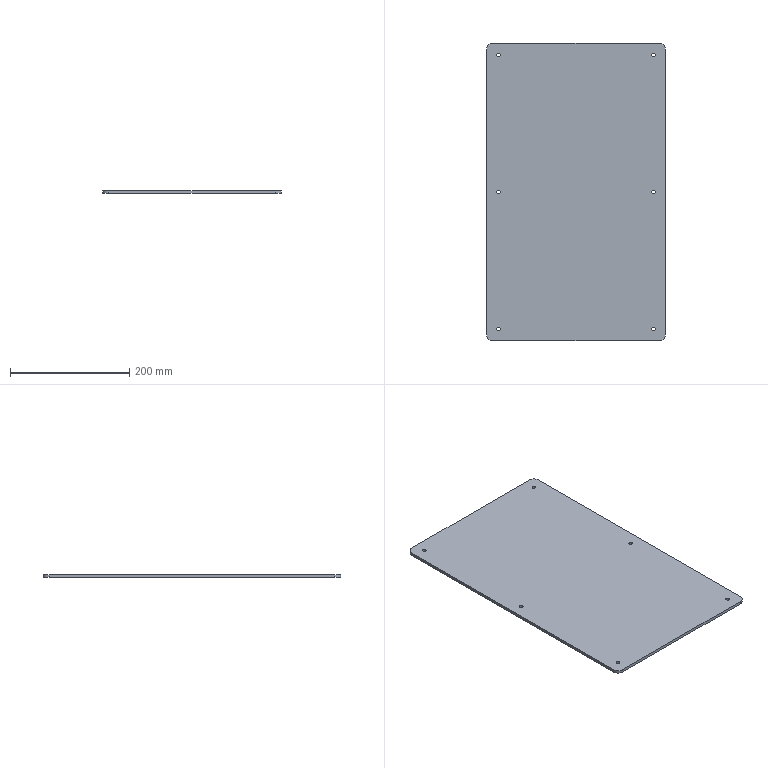Part | SolidWorks | features Extrusion 1, Fillet 1, HoleWzd 1 | 1 solid | 22 faces | box 300 x 500 x 5 mm | volume 748723 mm3 | cylinder 16 | plane 6 | commonest cylinder face diameters 6 x12 20 x4
STEP:
#1=CARTESIAN_POINT('',(-127.,230.,0.));
#2=VERTEX_POINT('',#1);
#3=CARTESIAN_POINT('',(-133.,230.,0.));
#4=VERTEX_POINT('',#3);
#5=CARTESIAN_POINT('',(-130.,230.,0.));
#6=DIRECTION('',(0.,0.,-1.));
#7=DIRECTION('',(-1.,0.,0.));
#8=AXIS2_PLACEMENT_3D('',#5,#6,#7);
#9=CIRCLE('',#8,3.);
#10=EDGE_CURVE('',#2,#4,#9,.T.);
#11=ORIENTED_EDGE('',*,*,#10,.T.);
#12=CARTESIAN_POINT('',(-133.,230.,5.));
#13=VERTEX_POINT('',#12);
#14=CARTESIAN_POINT('',(-133.,230.,5.));
#15=DIRECTION('',(0.,0.,1.));
#16=VECTOR('',#15,1000.);
#17=LINE('',#14,#16);
#18=EDGE_CURVE('',#4,#13,#17,.T.);
#19=ORIENTED_EDGE('',*,*,#18,.T.);
#20=CARTESIAN_POINT('',(-127.,230.,5.));
#21=VERTEX_POINT('',#20);
#22=CARTESIAN_POINT('',(-130.,230.,5.));
#23=DIRECTION('',(0.,0.,1.));
#24=DIRECTION('',(1.,0.,0.));
#25=AXIS2_PLACEMENT_3D('',#22,#23,#24);
#26=CIRCLE('',#25,3.);
#27=EDGE_CURVE('',#13,#21,#26,.T.);
#28=ORIENTED_EDGE('',*,*,#27,.T.);
#29=CARTESIAN_POINT('',(-127.,230.,5.));
#30=DIRECTION('',(0.,0.,1.));
#31=VECTOR('',#30,1000.);
#32=LINE('',#29,#31);
#33=EDGE_CURVE('',#2,#21,#32,.T.);
#34=ORIENTED_EDGE('',*,*,#33,.F.);
#35=EDGE_LOOP('',(#11,#19,#28,#34));
#36=FACE_OUTER_BOUND('',#35,.T.);
#37=CARTESIAN_POINT('',(-130.,230.,5.));
#38=DIRECTION('',(0.,0.,1.));
#39=DIRECTION('',(1.,0.,0.));
#40=AXIS2_PLACEMENT_3D('',#37,#38,#39);
#41=CYLINDRICAL_SURFACE('',#40,3.);
#42=ADVANCED_FACE('',(#36),#41,.F.);
#43=CARTESIAN_POINT('',(133.,230.,0.));
#44=VERTEX_POINT('',#43);
#45=CARTESIAN_POINT('',(127.,230.,0.));
#46=VERTEX_POINT('',#45);
#47=CARTESIAN_POINT('',(130.,230.,0.));
#48=DIRECTION('',(0.,0.,-1.));
#49=DIRECTION('',(-1.,0.,0.));
#50=AXIS2_PLACEMENT_3D('',#47,#48,#49);
#51=CIRCLE('',#50,3.);
#52=EDGE_CURVE('',#44,#46,#51,.T.);
#53=ORIENTED_EDGE('',*,*,#52,.T.);
#54=CARTESIAN_POINT('',(127.,230.,5.));
#55=VERTEX_POINT('',#54);
#56=CARTESIAN_POINT('',(127.,230.,5.));
#57=DIRECTION('',(0.,0.,1.));
#58=VECTOR('',#57,1000.);
#59=LINE('',#56,#58);
#60=EDGE_CURVE('',#46,#55,#59,.T.);
#61=ORIENTED_EDGE('',*,*,#60,.T.);
#62=CARTESIAN_POINT('',(133.,230.,5.));
#63=VERTEX_POINT('',#62);
#64=CARTESIAN_POINT('',(130.,230.,5.));
#65=DIRECTION('',(0.,0.,1.));
#66=DIRECTION('',(1.,0.,0.));
#67=AXIS2_PLACEMENT_3D('',#64,#65,#66);
#68=CIRCLE('',#67,3.);
#69=EDGE_CURVE('',#55,#63,#68,.T.);
#70=ORIENTED_EDGE('',*,*,#69,.T.);
#71=CARTESIAN_POINT('',(133.,230.,5.));
#72=DIRECTION('',(0.,0.,1.));
#73=VECTOR('',#72,1000.);
#74=LINE('',#71,#73);
#75=EDGE_CURVE('',#44,#63,#74,.T.);
#76=ORIENTED_EDGE('',*,*,#75,.F.);
#77=EDGE_LOOP('',(#53,#61,#70,#76));
#78=FACE_OUTER_BOUND('',#77,.T.);
#79=CARTESIAN_POINT('',(130.,230.,5.));
#80=DIRECTION('',(0.,0.,1.));
#81=DIRECTION('',(1.,0.,0.));
#82=AXIS2_PLACEMENT_3D('',#79,#80,#81);
#83=CYLINDRICAL_SURFACE('',#82,3.);
#84=ADVANCED_FACE('',(#78),#83,.F.);
#85=CARTESIAN_POINT('',(133.,-230.,0.));
#86=VERTEX_POINT('',#85);
#87=CARTESIAN_POINT('',(127.,-230.,0.));
#88=VERTEX_POINT('',#87);
#89=CARTESIAN_POINT('',(130.,-230.,0.));
#90=DIRECTION('',(0.,0.,-1.));
#91=DIRECTION('',(-1.,0.,0.));
#92=AXIS2_PLACEMENT_3D('',#89,#90,#91);
#93=CIRCLE('',#92,3.);
#94=EDGE_CURVE('',#86,#88,#93,.T.);
#95=ORIENTED_EDGE('',*,*,#94,.T.);
#96=CARTESIAN_POINT('',(127.,-230.,5.));
#97=VERTEX_POINT('',#96);
#98=CARTESIAN_POINT('',(127.,-230.,5.));
#99=DIRECTION('',(0.,0.,1.));
#100=VECTOR('',#99,1000.);
#101=LINE('',#98,#100);
#102=EDGE_CURVE('',#88,#97,#101,.T.);
#103=ORIENTED_EDGE('',*,*,#102,.T.);
#104=CARTESIAN_POINT('',(133.,-230.,5.));
#105=VERTEX_POINT('',#104);
#106=CARTESIAN_POINT('',(130.,-230.,5.));
#107=DIRECTION('',(0.,0.,1.));
#108=DIRECTION('',(1.,0.,0.));
#109=AXIS2_PLACEMENT_3D('',#106,#107,#108);
#110=CIRCLE('',#109,3.);
#111=EDGE_CURVE('',#97,#105,#110,.T.);
#112=ORIENTED_EDGE('',*,*,#111,.T.);
#113=CARTESIAN_POINT('',(133.,-230.,5.));
#114=DIRECTION('',(0.,0.,1.));
#115=VECTOR('',#114,1000.);
#116=LINE('',#113,#115);
#117=EDGE_CURVE('',#86,#105,#116,.T.);
#118=ORIENTED_EDGE('',*,*,#117,.F.);
#119=EDGE_LOOP('',(#95,#103,#112,#118));
#120=FACE_OUTER_BOUND('',#119,.T.);
#121=CARTESIAN_POINT('',(130.,-230.,5.));
#122=DIRECTION('',(0.,0.,1.));
#123=DIRECTION('',(1.,0.,0.));
#124=AXIS2_PLACEMENT_3D('',#121,#122,#123);
#125=CYLINDRICAL_SURFACE('',#124,3.);
#126=ADVANCED_FACE('',(#120),#125,.F.);
#127=CARTESIAN_POINT('',(-127.,-230.,0.));
#128=VERTEX_POINT('',#127);
#129=CARTESIAN_POINT('',(-133.,-230.,0.));
#130=VERTEX_POINT('',#129);
#131=CARTESIAN_POINT('',(-130.,-230.,0.));
#132=DIRECTION('',(0.,0.,-1.));
#133=DIRECTION('',(-1.,0.,0.));
#134=AXIS2_PLACEMENT_3D('',#131,#132,#133);
#135=CIRCLE('',#134,3.);
#136=EDGE_CURVE('',#128,#130,#135,.T.);
#137=ORIENTED_EDGE('',*,*,#136,.T.);
#138=CARTESIAN_POINT('',(-133.,-230.,5.));
#139=VERTEX_POINT('',#138);
#140=CARTESIAN_POINT('',(-133.,-230.,5.));
#141=DIRECTION('',(0.,0.,1.));
#142=VECTOR('',#141,1000.);
#143=LINE('',#140,#142);
#144=EDGE_CURVE('',#130,#139,#143,.T.);
#145=ORIENTED_EDGE('',*,*,#144,.T.);
#146=CARTESIAN_POINT('',(-127.,-230.,5.));
#147=VERTEX_POINT('',#146);
#148=CARTESIAN_POINT('',(-130.,-230.,5.));
#149=DIRECTION('',(0.,0.,1.));
#150=DIRECTION('',(1.,0.,0.));
#151=AXIS2_PLACEMENT_3D('',#148,#149,#150);
#152=CIRCLE('',#151,3.);
#153=EDGE_CURVE('',#139,#147,#152,.T.);
#154=ORIENTED_EDGE('',*,*,#153,.T.);
#155=CARTESIAN_POINT('',(-127.,-230.,5.));
#156=DIRECTION('',(0.,0.,1.));
#157=VECTOR('',#156,1000.);
#158=LINE('',#155,#157);
#159=EDGE_CURVE('',#128,#147,#158,.T.);
#160=ORIENTED_EDGE('',*,*,#159,.F.);
#161=EDGE_LOOP('',(#137,#145,#154,#160));
#162=FACE_OUTER_BOUND('',#161,.T.);
#163=CARTESIAN_POINT('',(-130.,-230.,5.));
#164=DIRECTION('',(0.,0.,1.));
#165=DIRECTION('',(1.,0.,0.));
#166=AXIS2_PLACEMENT_3D('',#163,#164,#165);
#167=CYLINDRICAL_SURFACE('',#166,3.);
#168=ADVANCED_FACE('',(#162),#167,.F.);
#169=CARTESIAN_POINT('',(-127.,0.,0.));
#170=VERTEX_POINT('',#169);
#171=CARTESIAN_POINT('',(-133.,0.,0.));
#172=VERTEX_POINT('',#171);
#173=CARTESIAN_POINT('',(-130.,0.,0.));
#174=DIRECTION('',(0.,0.,-1.));
#175=DIRECTION('',(-1.,0.,0.));
#176=AXIS2_PLACEMENT_3D('',#173,#174,#175);
#177=CIRCLE('',#176,3.);
#178=EDGE_CURVE('',#170,#172,#177,.T.);
#179=ORIENTED_EDGE('',*,*,#178,.T.);
#180=CARTESIAN_POINT('',(-133.,0.,5.));
#181=VERTEX_POINT('',#180);
#182=CARTESIAN_POINT('',(-133.,0.,5.));
#183=DIRECTION('',(0.,0.,1.));
#184=VECTOR('',#183,1000.);
#185=LINE('',#182,#184);
#186=EDGE_CURVE('',#172,#181,#185,.T.);
#187=ORIENTED_EDGE('',*,*,#186,.T.);
#188=CARTESIAN_POINT('',(-127.,0.,5.));
#189=VERTEX_POINT('',#188);
#190=CARTESIAN_POINT('',(-130.,0.,5.));
#191=DIRECTION('',(0.,0.,1.));
#192=DIRECTION('',(1.,0.,0.));
#193=AXIS2_PLACEMENT_3D('',#190,#191,#192);
#194=CIRCLE('',#193,3.);
#195=EDGE_CURVE('',#181,#189,#194,.T.);
#196=ORIENTED_EDGE('',*,*,#195,.T.);
#197=CARTESIAN_POINT('',(-127.,0.,5.));
#198=DIRECTION('',(0.,0.,1.));
#199=VECTOR('',#198,1000.);
#200=LINE('',#197,#199);
#201=EDGE_CURVE('',#170,#189,#200,.T.);
#202=ORIENTED_EDGE('',*,*,#201,.F.);
#203=EDGE_LOOP('',(#179,#187,#196,#202));
#204=FACE_OUTER_BOUND('',#203,.T.);
#205=CARTESIAN_POINT('',(-130.,0.,5.));
#206=DIRECTION('',(0.,0.,1.));
#207=DIRECTION('',(1.,0.,0.));
#208=AXIS2_PLACEMENT_3D('',#205,#206,#207);
#209=CYLINDRICAL_SURFACE('',#208,3.);
#210=ADVANCED_FACE('',(#204),#209,.F.);
#211=CARTESIAN_POINT('',(133.,0.,0.));
#212=VERTEX_POINT('',#211);
#213=CARTESIAN_POINT('',(127.,0.,0.));
#214=VERTEX_POINT('',#213);
#215=CARTESIAN_POINT('',(130.,0.,0.));
#216=DIRECTION('',(0.,0.,-1.));
#217=DIRECTION('',(-1.,0.,0.));
#218=AXIS2_PLACEMENT_3D('',#215,#216,#217);
#219=CIRCLE('',#218,3.);
#220=EDGE_CURVE('',#212,#214,#219,.T.);
#221=ORIENTED_EDGE('',*,*,#220,.T.);
#222=CARTESIAN_POINT('',(127.,0.,5.));
#223=VERTEX_POINT('',#222);
#224=CARTESIAN_POINT('',(127.,0.,5.));
#225=DIRECTION('',(0.,0.,1.));
#226=VECTOR('',#225,1000.);
#227=LINE('',#224,#226);
#228=EDGE_CURVE('',#214,#223,#227,.T.);
#229=ORIENTED_EDGE('',*,*,#228,.T.);
#230=CARTESIAN_POINT('',(133.,0.,5.));
#231=VERTEX_POINT('',#230);
#232=CARTESIAN_POINT('',(130.,0.,5.));
#233=DIRECTION('',(0.,0.,1.));
#234=DIRECTION('',(1.,0.,0.));
#235=AXIS2_PLACEMENT_3D('',#232,#233,#234);
#236=CIRCLE('',#235,3.);
#237=EDGE_CURVE('',#223,#231,#236,.T.);
#238=ORIENTED_EDGE('',*,*,#237,.T.);
#239=CARTESIAN_POINT('',(133.,0.,5.));
#240=DIRECTION('',(0.,0.,1.));
#241=VECTOR('',#240,1000.);
#242=LINE('',#239,#241);
#243=EDGE_CURVE('',#212,#231,#242,.T.);
#244=ORIENTED_EDGE('',*,*,#243,.F.);
#245=EDGE_LOOP('',(#221,#229,#238,#244));
#246=FACE_OUTER_BOUND('',#245,.T.);
#247=CARTESIAN_POINT('',(130.,0.,5.));
#248=DIRECTION('',(0.,0.,1.));
#249=DIRECTION('',(1.,0.,0.));
#250=AXIS2_PLACEMENT_3D('',#247,#248,#249);
#251=CYLINDRICAL_SURFACE('',#250,3.);
#252=ADVANCED_FACE('',(#246),#251,.F.);
#253=CARTESIAN_POINT('',(150.,-240.,5.));
#254=VERTEX_POINT('',#253);
#255=CARTESIAN_POINT('',(150.,240.,5.));
#256=VERTEX_POINT('',#255);
#257=CARTESIAN_POINT('',(150.,-250.,5.));
#258=DIRECTION('',(0.,1.,0.));
#259=VECTOR('',#258,1000.);
#260=LINE('',#257,#259);
#261=EDGE_CURVE('',#254,#256,#260,.T.);
#262=ORIENTED_EDGE('',*,*,#261,.F.);
#263=CARTESIAN_POINT('',(150.,-240.,0.));
#264=VERTEX_POINT('',#263);
#265=CARTESIAN_POINT('',(150.,-240.,5.));
#266=DIRECTION('',(0.,0.,-1.));
#267=VECTOR('',#266,1000.);
#268=LINE('',#265,#267);
#269=EDGE_CURVE('',#254,#264,#268,.T.);
#270=ORIENTED_EDGE('',*,*,#269,.T.);
#271=CARTESIAN_POINT('',(150.,240.,0.));
#272=VERTEX_POINT('',#271);
#273=CARTESIAN_POINT('',(150.,-250.,0.));
#274=DIRECTION('',(0.,1.,0.));
#275=VECTOR('',#274,1000.);
#276=LINE('',#273,#275);
#277=EDGE_CURVE('',#264,#272,#276,.T.);
#278=ORIENTED_EDGE('',*,*,#277,.T.);
#279=CARTESIAN_POINT('',(150.,240.,5.));
#280=DIRECTION('',(0.,0.,1.));
#281=VECTOR('',#280,1000.);
#282=LINE('',#279,#281);
#283=EDGE_CURVE('',#272,#256,#282,.T.);
#284=ORIENTED_EDGE('',*,*,#283,.T.);
#285=EDGE_LOOP('',(#262,#270,#278,#284));
#286=FACE_OUTER_BOUND('',#285,.T.);
#287=CARTESIAN_POINT('',(150.,-250.,5.));
#288=DIRECTION('',(-1.,0.,0.));
#289=DIRECTION('',(0.,0.,1.));
#290=AXIS2_PLACEMENT_3D('',#287,#288,#289);
#291=PLANE('',#290);
#292=ADVANCED_FACE('',(#286),#291,.F.);
#293=CARTESIAN_POINT('',(140.,250.,5.));
#294=VERTEX_POINT('',#293);
#295=CARTESIAN_POINT('',(-140.,250.,5.));
#296=VERTEX_POINT('',#295);
#297=CARTESIAN_POINT('',(-150.,250.,5.));
#298=DIRECTION('',(-1.,0.,0.));
#299=VECTOR('',#298,1000.);
#300=LINE('',#297,#299);
#301=EDGE_CURVE('',#294,#296,#300,.T.);
#302=ORIENTED_EDGE('',*,*,#301,.F.);
#303=CARTESIAN_POINT('',(140.,250.,0.));
#304=VERTEX_POINT('',#303);
#305=CARTESIAN_POINT('',(140.,250.,5.));
#306=DIRECTION('',(0.,0.,-1.));
#307=VECTOR('',#306,1000.);
#308=LINE('',#305,#307);
#309=EDGE_CURVE('',#294,#304,#308,.T.);
#310=ORIENTED_EDGE('',*,*,#309,.T.);
#311=CARTESIAN_POINT('',(-140.,250.,0.));
#312=VERTEX_POINT('',#311);
#313=CARTESIAN_POINT('',(-150.,250.,0.));
#314=DIRECTION('',(-1.,0.,0.));
#315=VECTOR('',#314,1000.);
#316=LINE('',#313,#315);
#317=EDGE_CURVE('',#304,#312,#316,.T.);
#318=ORIENTED_EDGE('',*,*,#317,.T.);
#319=CARTESIAN_POINT('',(-140.,250.,5.));
#320=DIRECTION('',(0.,0.,1.));
#321=VECTOR('',#320,1000.);
#322=LINE('',#319,#321);
#323=EDGE_CURVE('',#312,#296,#322,.T.);
#324=ORIENTED_EDGE('',*,*,#323,.T.);
#325=EDGE_LOOP('',(#302,#310,#318,#324));
#326=FACE_OUTER_BOUND('',#325,.T.);
#327=CARTESIAN_POINT('',(-150.,250.,5.));
#328=DIRECTION('',(0.,-1.,0.));
#329=DIRECTION('',(0.,0.,-1.));
#330=AXIS2_PLACEMENT_3D('',#327,#328,#329);
#331=PLANE('',#330);
#332=ADVANCED_FACE('',(#326),#331,.F.);
#333=CARTESIAN_POINT('',(-150.,240.,0.));
#334=VERTEX_POINT('',#333);
#335=CARTESIAN_POINT('',(-150.,-240.,0.));
#336=VERTEX_POINT('',#335);
#337=CARTESIAN_POINT('',(-150.,-250.,0.));
#338=DIRECTION('',(0.,-1.,0.));
#339=VECTOR('',#338,1000.);
#340=LINE('',#337,#339);
#341=EDGE_CURVE('',#334,#336,#340,.T.);
#342=ORIENTED_EDGE('',*,*,#341,.T.);
#343=CARTESIAN_POINT('',(-150.,-240.,5.));
#344=VERTEX_POINT('',#343);
#345=CARTESIAN_POINT('',(-150.,-240.,5.));
#346=DIRECTION('',(0.,0.,1.));
#347=VECTOR('',#346,1000.);
#348=LINE('',#345,#347);
#349=EDGE_CURVE('',#336,#344,#348,.T.);
#350=ORIENTED_EDGE('',*,*,#349,.T.);
#351=CARTESIAN_POINT('',(-150.,240.,5.));
#352=VERTEX_POINT('',#351);
#353=CARTESIAN_POINT('',(-150.,-250.,5.));
#354=DIRECTION('',(0.,-1.,0.));
#355=VECTOR('',#354,1000.);
#356=LINE('',#353,#355);
#357=EDGE_CURVE('',#352,#344,#356,.T.);
#358=ORIENTED_EDGE('',*,*,#357,.F.);
#359=CARTESIAN_POINT('',(-150.,240.,5.));
#360=DIRECTION('',(0.,0.,-1.));
#361=VECTOR('',#360,1000.);
#362=LINE('',#359,#361);
#363=EDGE_CURVE('',#352,#334,#362,.T.);
#364=ORIENTED_EDGE('',*,*,#363,.T.);
#365=EDGE_LOOP('',(#342,#350,#358,#364));
#366=FACE_OUTER_BOUND('',#365,.T.);
#367=CARTESIAN_POINT('',(-150.,-250.,5.));
#368=DIRECTION('',(1.,0.,0.));
#369=DIRECTION('',(0.,0.,-1.));
#370=AXIS2_PLACEMENT_3D('',#367,#368,#369);
#371=PLANE('',#370);
#372=ADVANCED_FACE('',(#366),#371,.F.);
#373=CARTESIAN_POINT('',(-140.,-250.,5.));
#374=VERTEX_POINT('',#373);
#375=CARTESIAN_POINT('',(140.,-250.,5.));
#376=VERTEX_POINT('',#375);
#377=CARTESIAN_POINT('',(-150.,-250.,5.));
#378=DIRECTION('',(1.,0.,0.));
#379=VECTOR('',#378,1000.);
#380=LINE('',#377,#379);
#381=EDGE_CURVE('',#374,#376,#380,.T.);
#382=ORIENTED_EDGE('',*,*,#381,.F.);
#383=CARTESIAN_POINT('',(-140.,-250.,0.));
#384=VERTEX_POINT('',#383);
#385=CARTESIAN_POINT('',(-140.,-250.,5.));
#386=DIRECTION('',(0.,0.,-1.));
#387=VECTOR('',#386,1000.);
#388=LINE('',#385,#387);
#389=EDGE_CURVE('',#374,#384,#388,.T.);
#390=ORIENTED_EDGE('',*,*,#389,.T.);
#391=CARTESIAN_POINT('',(140.,-250.,0.));
#392=VERTEX_POINT('',#391);
#393=CARTESIAN_POINT('',(-150.,-250.,0.));
#394=DIRECTION('',(1.,0.,0.));
#395=VECTOR('',#394,1000.);
#396=LINE('',#393,#395);
#397=EDGE_CURVE('',#384,#392,#396,.T.);
#398=ORIENTED_EDGE('',*,*,#397,.T.);
#399=CARTESIAN_POINT('',(140.,-250.,5.));
#400=DIRECTION('',(0.,0.,1.));
#401=VECTOR('',#400,1000.);
#402=LINE('',#399,#401);
#403=EDGE_CURVE('',#392,#376,#402,.T.);
#404=ORIENTED_EDGE('',*,*,#403,.T.);
#405=EDGE_LOOP('',(#382,#390,#398,#404));
#406=FACE_OUTER_BOUND('',#405,.T.);
#407=CARTESIAN_POINT('',(-150.,-250.,5.));
#408=DIRECTION('',(0.,1.,0.));
#409=DIRECTION('',(0.,0.,1.));
#410=AXIS2_PLACEMENT_3D('',#407,#408,#409);
#411=PLANE('',#410);
#412=ADVANCED_FACE('',(#406),#411,.F.);
#413=CARTESIAN_POINT('',(-130.,230.,5.));
#414=DIRECTION('',(0.,0.,1.));
#415=DIRECTION('',(1.,0.,0.));
#416=AXIS2_PLACEMENT_3D('',#413,#414,#415);
#417=CIRCLE('',#416,3.);
#418=EDGE_CURVE('',#21,#13,#417,.T.);
#419=ORIENTED_EDGE('',*,*,#418,.F.);
#420=ORIENTED_EDGE('',*,*,#27,.F.);
#421=EDGE_LOOP('',(#419,#420));
#422=FACE_BOUND('',#421,.T.);
#423=CARTESIAN_POINT('',(130.,230.,5.));
#424=DIRECTION('',(0.,0.,1.));
#425=DIRECTION('',(1.,0.,0.));
#426=AXIS2_PLACEMENT_3D('',#423,#424,#425);
#427=CIRCLE('',#426,3.);
#428=EDGE_CURVE('',#63,#55,#427,.T.);
#429=ORIENTED_EDGE('',*,*,#428,.F.);
#430=ORIENTED_EDGE('',*,*,#69,.F.);
#431=EDGE_LOOP('',(#429,#430));
#432=FACE_BOUND('',#431,.T.);
#433=CARTESIAN_POINT('',(130.,-230.,5.));
#434=DIRECTION('',(0.,0.,1.));
#435=DIRECTION('',(1.,0.,0.));
#436=AXIS2_PLACEMENT_3D('',#433,#434,#435);
#437=CIRCLE('',#436,3.);
#438=EDGE_CURVE('',#105,#97,#437,.T.);
#439=ORIENTED_EDGE('',*,*,#438,.F.);
#440=ORIENTED_EDGE('',*,*,#111,.F.);
#441=EDGE_LOOP('',(#439,#440));
#442=FACE_BOUND('',#441,.T.);
#443=CARTESIAN_POINT('',(-130.,-230.,5.));
#444=DIRECTION('',(0.,0.,1.));
#445=DIRECTION('',(1.,0.,0.));
#446=AXIS2_PLACEMENT_3D('',#443,#444,#445);
#447=CIRCLE('',#446,3.);
#448=EDGE_CURVE('',#147,#139,#447,.T.);
#449=ORIENTED_EDGE('',*,*,#448,.F.);
#450=ORIENTED_EDGE('',*,*,#153,.F.);
#451=EDGE_LOOP('',(#449,#450));
#452=FACE_BOUND('',#451,.T.);
#453=CARTESIAN_POINT('',(-130.,0.,5.));
#454=DIRECTION('',(0.,0.,1.));
#455=DIRECTION('',(1.,0.,0.));
#456=AXIS2_PLACEMENT_3D('',#453,#454,#455);
#457=CIRCLE('',#456,3.);
#458=EDGE_CURVE('',#189,#181,#457,.T.);
#459=ORIENTED_EDGE('',*,*,#458,.F.);
#460=ORIENTED_EDGE('',*,*,#195,.F.);
#461=EDGE_LOOP('',(#459,#460));
#462=FACE_BOUND('',#461,.T.);
#463=CARTESIAN_POINT('',(130.,0.,5.));
#464=DIRECTION('',(0.,0.,1.));
#465=DIRECTION('',(1.,0.,0.));
#466=AXIS2_PLACEMENT_3D('',#463,#464,#465);
#467=CIRCLE('',#466,3.);
#468=EDGE_CURVE('',#231,#223,#467,.T.);
#469=ORIENTED_EDGE('',*,*,#468,.F.);
#470=ORIENTED_EDGE('',*,*,#237,.F.);
#471=EDGE_LOOP('',(#469,#470));
#472=FACE_BOUND('',#471,.T.);
#473=ORIENTED_EDGE('',*,*,#357,.T.);
#474=CARTESIAN_POINT('',(-140.,-240.,5.));
#475=DIRECTION('',(0.,0.,1.));
#476=DIRECTION('',(-1.,0.,0.));
#477=AXIS2_PLACEMENT_3D('',#474,#475,#476);
#478=CIRCLE('',#477,10.);
#479=EDGE_CURVE('',#344,#374,#478,.T.);
#480=ORIENTED_EDGE('',*,*,#479,.T.);
#481=ORIENTED_EDGE('',*,*,#381,.T.);
#482=CARTESIAN_POINT('',(140.,-240.,5.));
#483=DIRECTION('',(0.,0.,1.));
#484=DIRECTION('',(-1.,0.,0.));
#485=AXIS2_PLACEMENT_3D('',#482,#483,#484);
#486=CIRCLE('',#485,10.);
#487=EDGE_CURVE('',#376,#254,#486,.T.);
#488=ORIENTED_EDGE('',*,*,#487,.T.);
#489=ORIENTED_EDGE('',*,*,#261,.T.);
#490=CARTESIAN_POINT('',(140.,240.,5.));
#491=DIRECTION('',(0.,0.,1.));
#492=DIRECTION('',(-1.,0.,0.));
#493=AXIS2_PLACEMENT_3D('',#490,#491,#492);
#494=CIRCLE('',#493,10.);
#495=EDGE_CURVE('',#256,#294,#494,.T.);
#496=ORIENTED_EDGE('',*,*,#495,.T.);
#497=ORIENTED_EDGE('',*,*,#301,.T.);
#498=CARTESIAN_POINT('',(-140.,240.,5.));
#499=DIRECTION('',(0.,0.,1.));
#500=DIRECTION('',(-1.,0.,0.));
#501=AXIS2_PLACEMENT_3D('',#498,#499,#500);
#502=CIRCLE('',#501,10.);
#503=EDGE_CURVE('',#296,#352,#502,.T.);
#504=ORIENTED_EDGE('',*,*,#503,.T.);
#505=EDGE_LOOP('',(#473,#480,#481,#488,#489,#496,#497,#504));
#506=FACE_OUTER_BOUND('',#505,.T.);
#507=CARTESIAN_POINT('',(0.,0.,5.));
#508=DIRECTION('',(0.,0.,-1.));
#509=DIRECTION('',(-1.,0.,0.));
#510=AXIS2_PLACEMENT_3D('',#507,#508,#509);
#511=PLANE('',#510);
#512=ADVANCED_FACE('',(#422,#432,#442,#452,#462,#472,#506),#511,.F.);
#513=ORIENTED_EDGE('',*,*,#10,.F.);
#514=CARTESIAN_POINT('',(-130.,230.,0.));
#515=DIRECTION('',(0.,0.,-1.));
#516=DIRECTION('',(-1.,0.,0.));
#517=AXIS2_PLACEMENT_3D('',#514,#515,#516);
#518=CIRCLE('',#517,3.);
#519=EDGE_CURVE('',#4,#2,#518,.T.);
#520=ORIENTED_EDGE('',*,*,#519,.F.);
#521=EDGE_LOOP('',(#513,#520));
#522=FACE_BOUND('',#521,.T.);
#523=ORIENTED_EDGE('',*,*,#52,.F.);
#524=CARTESIAN_POINT('',(130.,230.,0.));
#525=DIRECTION('',(0.,0.,-1.));
#526=DIRECTION('',(-1.,0.,0.));
#527=AXIS2_PLACEMENT_3D('',#524,#525,#526);
#528=CIRCLE('',#527,3.);
#529=EDGE_CURVE('',#46,#44,#528,.T.);
#530=ORIENTED_EDGE('',*,*,#529,.F.);
#531=EDGE_LOOP('',(#523,#530));
#532=FACE_BOUND('',#531,.T.);
#533=ORIENTED_EDGE('',*,*,#94,.F.);
#534=CARTESIAN_POINT('',(130.,-230.,0.));
#535=DIRECTION('',(0.,0.,-1.));
#536=DIRECTION('',(-1.,0.,0.));
#537=AXIS2_PLACEMENT_3D('',#534,#535,#536);
#538=CIRCLE('',#537,3.);
#539=EDGE_CURVE('',#88,#86,#538,.T.);
#540=ORIENTED_EDGE('',*,*,#539,.F.);
#541=EDGE_LOOP('',(#533,#540));
#542=FACE_BOUND('',#541,.T.);
#543=ORIENTED_EDGE('',*,*,#136,.F.);
#544=CARTESIAN_POINT('',(-130.,-230.,0.));
#545=DIRECTION('',(0.,0.,-1.));
#546=DIRECTION('',(-1.,0.,0.));
#547=AXIS2_PLACEMENT_3D('',#544,#545,#546);
#548=CIRCLE('',#547,3.);
#549=EDGE_CURVE('',#130,#128,#548,.T.);
#550=ORIENTED_EDGE('',*,*,#549,.F.);
#551=EDGE_LOOP('',(#543,#550));
#552=FACE_BOUND('',#551,.T.);
#553=ORIENTED_EDGE('',*,*,#178,.F.);
#554=CARTESIAN_POINT('',(-130.,0.,0.));
#555=DIRECTION('',(0.,0.,-1.));
#556=DIRECTION('',(-1.,0.,0.));
#557=AXIS2_PLACEMENT_3D('',#554,#555,#556);
#558=CIRCLE('',#557,3.);
#559=EDGE_CURVE('',#172,#170,#558,.T.);
#560=ORIENTED_EDGE('',*,*,#559,.F.);
#561=EDGE_LOOP('',(#553,#560));
#562=FACE_BOUND('',#561,.T.);
#563=ORIENTED_EDGE('',*,*,#220,.F.);
#564=CARTESIAN_POINT('',(130.,0.,0.));
#565=DIRECTION('',(0.,0.,-1.));
#566=DIRECTION('',(-1.,0.,0.));
#567=AXIS2_PLACEMENT_3D('',#564,#565,#566);
#568=CIRCLE('',#567,3.);
#569=EDGE_CURVE('',#214,#212,#568,.T.);
#570=ORIENTED_EDGE('',*,*,#569,.F.);
#571=EDGE_LOOP('',(#563,#570));
#572=FACE_BOUND('',#571,.T.);
#573=ORIENTED_EDGE('',*,*,#397,.F.);
#574=CARTESIAN_POINT('',(-140.,-240.,0.));
#575=DIRECTION('',(0.,0.,-1.));
#576=DIRECTION('',(-1.,0.,0.));
#577=AXIS2_PLACEMENT_3D('',#574,#575,#576);
#578=CIRCLE('',#577,10.);
#579=EDGE_CURVE('',#384,#336,#578,.T.);
#580=ORIENTED_EDGE('',*,*,#579,.T.);
#581=ORIENTED_EDGE('',*,*,#341,.F.);
#582=CARTESIAN_POINT('',(-140.,240.,0.));
#583=DIRECTION('',(0.,0.,-1.));
#584=DIRECTION('',(-1.,0.,0.));
#585=AXIS2_PLACEMENT_3D('',#582,#583,#584);
#586=CIRCLE('',#585,10.);
#587=EDGE_CURVE('',#334,#312,#586,.T.);
#588=ORIENTED_EDGE('',*,*,#587,.T.);
#589=ORIENTED_EDGE('',*,*,#317,.F.);
#590=CARTESIAN_POINT('',(140.,240.,0.));
#591=DIRECTION('',(0.,0.,-1.));
#592=DIRECTION('',(-1.,0.,0.));
#593=AXIS2_PLACEMENT_3D('',#590,#591,#592);
#594=CIRCLE('',#593,10.);
#595=EDGE_CURVE('',#304,#272,#594,.T.);
#596=ORIENTED_EDGE('',*,*,#595,.T.);
#597=ORIENTED_EDGE('',*,*,#277,.F.);
#598=CARTESIAN_POINT('',(140.,-240.,0.));
#599=DIRECTION('',(0.,0.,-1.));
#600=DIRECTION('',(-1.,0.,0.));
#601=AXIS2_PLACEMENT_3D('',#598,#599,#600);
#602=CIRCLE('',#601,10.);
#603=EDGE_CURVE('',#264,#392,#602,.T.);
#604=ORIENTED_EDGE('',*,*,#603,.T.);
#605=EDGE_LOOP('',(#573,#580,#581,#588,#589,#596,#597,#604));
#606=FACE_OUTER_BOUND('',#605,.T.);
#607=CARTESIAN_POINT('',(0.,0.,0.));
#608=DIRECTION('',(0.,0.,-1.));
#609=DIRECTION('',(-1.,0.,0.));
#610=AXIS2_PLACEMENT_3D('',#607,#608,#609);
#611=PLANE('',#610);
#612=ADVANCED_FACE('',(#522,#532,#542,#552,#562,#572,#606),#611,.T.);
#613=ORIENTED_EDGE('',*,*,#228,.F.);
#614=ORIENTED_EDGE('',*,*,#569,.T.);
#615=ORIENTED_EDGE('',*,*,#243,.T.);
#616=ORIENTED_EDGE('',*,*,#468,.T.);
#617=EDGE_LOOP('',(#613,#614,#615,#616));
#618=FACE_OUTER_BOUND('',#617,.T.);
#619=CARTESIAN_POINT('',(130.,0.,5.));
#620=DIRECTION('',(0.,0.,1.));
#621=DIRECTION('',(1.,0.,0.));
#622=AXIS2_PLACEMENT_3D('',#619,#620,#621);
#623=CYLINDRICAL_SURFACE('',#622,3.);
#624=ADVANCED_FACE('',(#618),#623,.F.);
#625=ORIENTED_EDGE('',*,*,#186,.F.);
#626=ORIENTED_EDGE('',*,*,#559,.T.);
#627=ORIENTED_EDGE('',*,*,#201,.T.);
#628=ORIENTED_EDGE('',*,*,#458,.T.);
#629=EDGE_LOOP('',(#625,#626,#627,#628));
#630=FACE_OUTER_BOUND('',#629,.T.);
#631=CARTESIAN_POINT('',(-130.,0.,5.));
#632=DIRECTION('',(0.,0.,1.));
#633=DIRECTION('',(1.,0.,0.));
#634=AXIS2_PLACEMENT_3D('',#631,#632,#633);
#635=CYLINDRICAL_SURFACE('',#634,3.);
#636=ADVANCED_FACE('',(#630),#635,.F.);
#637=ORIENTED_EDGE('',*,*,#144,.F.);
#638=ORIENTED_EDGE('',*,*,#549,.T.);
#639=ORIENTED_EDGE('',*,*,#159,.T.);
#640=ORIENTED_EDGE('',*,*,#448,.T.);
#641=EDGE_LOOP('',(#637,#638,#639,#640));
#642=FACE_OUTER_BOUND('',#641,.T.);
#643=CARTESIAN_POINT('',(-130.,-230.,5.));
#644=DIRECTION('',(0.,0.,1.));
#645=DIRECTION('',(1.,0.,0.));
#646=AXIS2_PLACEMENT_3D('',#643,#644,#645);
#647=CYLINDRICAL_SURFACE('',#646,3.);
#648=ADVANCED_FACE('',(#642),#647,.F.);
#649=ORIENTED_EDGE('',*,*,#102,.F.);
#650=ORIENTED_EDGE('',*,*,#539,.T.);
#651=ORIENTED_EDGE('',*,*,#117,.T.);
#652=ORIENTED_EDGE('',*,*,#438,.T.);
#653=EDGE_LOOP('',(#649,#650,#651,#652));
#654=FACE_OUTER_BOUND('',#653,.T.);
#655=CARTESIAN_POINT('',(130.,-230.,5.));
#656=DIRECTION('',(0.,0.,1.));
#657=DIRECTION('',(1.,0.,0.));
#658=AXIS2_PLACEMENT_3D('',#655,#656,#657);
#659=CYLINDRICAL_SURFACE('',#658,3.);
#660=ADVANCED_FACE('',(#654),#659,.F.);
#661=ORIENTED_EDGE('',*,*,#60,.F.);
#662=ORIENTED_EDGE('',*,*,#529,.T.);
#663=ORIENTED_EDGE('',*,*,#75,.T.);
#664=ORIENTED_EDGE('',*,*,#428,.T.);
#665=EDGE_LOOP('',(#661,#662,#663,#664));
#666=FACE_OUTER_BOUND('',#665,.T.);
#667=CARTESIAN_POINT('',(130.,230.,5.));
#668=DIRECTION('',(0.,0.,1.));
#669=DIRECTION('',(1.,0.,0.));
#670=AXIS2_PLACEMENT_3D('',#667,#668,#669);
#671=CYLINDRICAL_SURFACE('',#670,3.);
#672=ADVANCED_FACE('',(#666),#671,.F.);
#673=ORIENTED_EDGE('',*,*,#18,.F.);
#674=ORIENTED_EDGE('',*,*,#519,.T.);
#675=ORIENTED_EDGE('',*,*,#33,.T.);
#676=ORIENTED_EDGE('',*,*,#418,.T.);
#677=EDGE_LOOP('',(#673,#674,#675,#676));
#678=FACE_OUTER_BOUND('',#677,.T.);
#679=CARTESIAN_POINT('',(-130.,230.,5.));
#680=DIRECTION('',(0.,0.,1.));
#681=DIRECTION('',(1.,0.,0.));
#682=AXIS2_PLACEMENT_3D('',#679,#680,#681);
#683=CYLINDRICAL_SURFACE('',#682,3.);
#684=ADVANCED_FACE('',(#678),#683,.F.);
#685=ORIENTED_EDGE('',*,*,#479,.F.);
#686=ORIENTED_EDGE('',*,*,#349,.F.);
#687=ORIENTED_EDGE('',*,*,#579,.F.);
#688=ORIENTED_EDGE('',*,*,#389,.F.);
#689=EDGE_LOOP('',(#685,#686,#687,#688));
#690=FACE_OUTER_BOUND('',#689,.T.);
#691=CARTESIAN_POINT('',(-140.,-240.,5.));
#692=DIRECTION('',(0.,0.,-1.));
#693=DIRECTION('',(-1.,0.,0.));
#694=AXIS2_PLACEMENT_3D('',#691,#692,#693);
#695=CYLINDRICAL_SURFACE('',#694,10.);
#696=ADVANCED_FACE('',(#690),#695,.T.);
#697=ORIENTED_EDGE('',*,*,#487,.F.);
#698=ORIENTED_EDGE('',*,*,#403,.F.);
#699=ORIENTED_EDGE('',*,*,#603,.F.);
#700=ORIENTED_EDGE('',*,*,#269,.F.);
#701=EDGE_LOOP('',(#697,#698,#699,#700));
#702=FACE_OUTER_BOUND('',#701,.T.);
#703=CARTESIAN_POINT('',(140.,-240.,5.));
#704=DIRECTION('',(0.,0.,-1.));
#705=DIRECTION('',(-1.,0.,0.));
#706=AXIS2_PLACEMENT_3D('',#703,#704,#705);
#707=CYLINDRICAL_SURFACE('',#706,10.);
#708=ADVANCED_FACE('',(#702),#707,.T.);
#709=ORIENTED_EDGE('',*,*,#495,.F.);
#710=ORIENTED_EDGE('',*,*,#283,.F.);
#711=ORIENTED_EDGE('',*,*,#595,.F.);
#712=ORIENTED_EDGE('',*,*,#309,.F.);
#713=EDGE_LOOP('',(#709,#710,#711,#712));
#714=FACE_OUTER_BOUND('',#713,.T.);
#715=CARTESIAN_POINT('',(140.,240.,5.));
#716=DIRECTION('',(0.,0.,-1.));
#717=DIRECTION('',(-1.,0.,0.));
#718=AXIS2_PLACEMENT_3D('',#715,#716,#717);
#719=CYLINDRICAL_SURFACE('',#718,10.);
#720=ADVANCED_FACE('',(#714),#719,.T.);
#721=ORIENTED_EDGE('',*,*,#503,.F.);
#722=ORIENTED_EDGE('',*,*,#323,.F.);
#723=ORIENTED_EDGE('',*,*,#587,.F.);
#724=ORIENTED_EDGE('',*,*,#363,.F.);
#725=EDGE_LOOP('',(#721,#722,#723,#724));
#726=FACE_OUTER_BOUND('',#725,.T.);
#727=CARTESIAN_POINT('',(-140.,240.,5.));
#728=DIRECTION('',(0.,0.,-1.));
#729=DIRECTION('',(-1.,0.,0.));
#730=AXIS2_PLACEMENT_3D('',#727,#728,#729);
#731=CYLINDRICAL_SURFACE('',#730,10.);
#732=ADVANCED_FACE('',(#726),#731,.T.);
#733=CLOSED_SHELL('',(#42,#84,#126,#168,#210,#252,#292,#332,#372,#412,#512,#612,#624,#636,#648,#660,#672,#684,#696,#708,#720,#732));
#734=MANIFOLD_SOLID_BREP('',#733);
#735=CARTESIAN_POINT('',(0.,0.,0.));
#736=DIRECTION('',(0.,0.,1.));
#737=DIRECTION('',(1.,0.,0.));
#738=AXIS2_PLACEMENT_3D('',#735,#736,#737);
#739=(LENGTH_UNIT()NAMED_UNIT(*)SI_UNIT(.MILLI.,.METRE.));
#740=UNCERTAINTY_MEASURE_WITH_UNIT(LENGTH_MEASURE(0.00001),#739,'','');
#741=(NAMED_UNIT(*)PLANE_ANGLE_UNIT()SI_UNIT($,.RADIAN.));
#742=(NAMED_UNIT(*)SI_UNIT($,.STERADIAN.)SOLID_ANGLE_UNIT());
#743=(GEOMETRIC_REPRESENTATION_CONTEXT(3)GLOBAL_UNCERTAINTY_ASSIGNED_CONTEXT((#740))GLOBAL_UNIT_ASSIGNED_CONTEXT((#739,#741,#742))REPRESENTATION_CONTEXT('',''));
#744=ADVANCED_BREP_SHAPE_REPRESENTATION('',(#734,#738),#743);